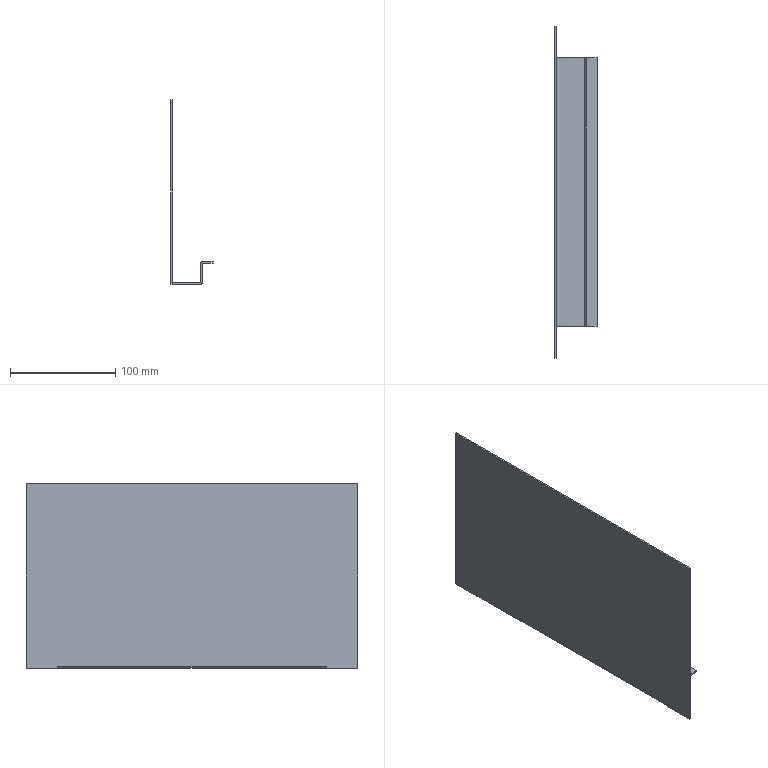Part | 1 solid | 38 faces | box 40 x 315 x 175 mm | volume 104644 mm3 | plane 32 | cylinder 6 | commonest cylinder face diameters 0.2 x3 3.2 x3
STEP:
#1=CARTESIAN_POINT('',(-217.5,127.5,-155.));
#2=VERTEX_POINT('',#1);
#3=CARTESIAN_POINT('',(-217.5,127.5,-153.5));
#4=VERTEX_POINT('',#3);
#5=CARTESIAN_POINT('',(-217.5,127.5,-663.884));
#6=DIRECTION('',(0.,0.,1.));
#7=VECTOR('',#6,1000.);
#8=LINE('',#5,#7);
#9=EDGE_CURVE('',#2,#4,#8,.T.);
#10=ORIENTED_EDGE('',*,*,#9,.T.);
#11=CARTESIAN_POINT('',(-217.5,-127.5,-153.5));
#12=VERTEX_POINT('',#11);
#13=CARTESIAN_POINT('',(-217.5,-127.5,-153.5));
#14=DIRECTION('',(0.,-1.,0.));
#15=VECTOR('',#14,1000.);
#16=LINE('',#13,#15);
#17=EDGE_CURVE('',#4,#12,#16,.T.);
#18=ORIENTED_EDGE('',*,*,#17,.T.);
#19=CARTESIAN_POINT('',(-217.5,-127.5,-155.));
#20=VERTEX_POINT('',#19);
#21=CARTESIAN_POINT('',(-217.5,-127.5,-663.884));
#22=DIRECTION('',(0.,0.,1.));
#23=VECTOR('',#22,1000.);
#24=LINE('',#21,#23);
#25=EDGE_CURVE('',#20,#12,#24,.T.);
#26=ORIENTED_EDGE('',*,*,#25,.F.);
#27=CARTESIAN_POINT('',(-217.5,-127.5,-155.));
#28=DIRECTION('',(0.,-1.,0.));
#29=VECTOR('',#28,1000.);
#30=LINE('',#27,#29);
#31=EDGE_CURVE('',#2,#20,#30,.T.);
#32=ORIENTED_EDGE('',*,*,#31,.F.);
#33=EDGE_LOOP('',(#10,#18,#26,#32));
#34=FACE_OUTER_BOUND('',#33,.T.);
#35=CARTESIAN_POINT('',(-217.5,-127.5,-663.884));
#36=DIRECTION('',(-1.,0.,0.));
#37=DIRECTION('',(0.,-1.,0.));
#38=AXIS2_PLACEMENT_3D('',#35,#36,#37);
#39=PLANE('',#38);
#40=ADVANCED_FACE('',(#34),#39,.F.);
#41=CARTESIAN_POINT('',(-227.4,127.5,-153.5));
#42=VERTEX_POINT('',#41);
#43=CARTESIAN_POINT('',(-2832.5,127.5,-153.5));
#44=DIRECTION('',(-1.,0.,0.));
#45=VECTOR('',#44,1000.);
#46=LINE('',#43,#45);
#47=EDGE_CURVE('',#4,#42,#46,.T.);
#48=ORIENTED_EDGE('',*,*,#47,.F.);
#49=ORIENTED_EDGE('',*,*,#9,.F.);
#50=CARTESIAN_POINT('',(-227.4,127.5,-155.));
#51=VERTEX_POINT('',#50);
#52=CARTESIAN_POINT('',(2832.5,127.5,-155.));
#53=DIRECTION('',(-1.,0.,0.));
#54=VECTOR('',#53,1000.);
#55=LINE('',#52,#54);
#56=EDGE_CURVE('',#2,#51,#55,.T.);
#57=ORIENTED_EDGE('',*,*,#56,.T.);
#58=CARTESIAN_POINT('',(-227.4,127.5,-663.884));
#59=DIRECTION('',(0.,0.,1.));
#60=VECTOR('',#59,1000.);
#61=LINE('',#58,#60);
#62=EDGE_CURVE('',#51,#42,#61,.T.);
#63=ORIENTED_EDGE('',*,*,#62,.T.);
#64=EDGE_LOOP('',(#48,#49,#57,#63));
#65=FACE_OUTER_BOUND('',#64,.T.);
#66=CARTESIAN_POINT('',(2832.5,127.5,-663.884));
#67=DIRECTION('',(0.,1.,0.));
#68=DIRECTION('',(-1.,0.,0.));
#69=AXIS2_PLACEMENT_3D('',#66,#67,#68);
#70=PLANE('',#69);
#71=ADVANCED_FACE('',(#65),#70,.T.);
#72=ORIENTED_EDGE('',*,*,#47,.T.);
#73=CARTESIAN_POINT('',(-227.4,-127.5,-153.5));
#74=VERTEX_POINT('',#73);
#75=CARTESIAN_POINT('',(-227.4,127.5,-153.5));
#76=DIRECTION('',(0.,-1.,0.));
#77=VECTOR('',#76,1000.);
#78=LINE('',#75,#77);
#79=EDGE_CURVE('',#42,#74,#78,.T.);
#80=ORIENTED_EDGE('',*,*,#79,.T.);
#81=CARTESIAN_POINT('',(-2832.5,-127.5,-153.5));
#82=DIRECTION('',(1.,0.,0.));
#83=VECTOR('',#82,1000.);
#84=LINE('',#81,#83);
#85=EDGE_CURVE('',#74,#12,#84,.T.);
#86=ORIENTED_EDGE('',*,*,#85,.T.);
#87=ORIENTED_EDGE('',*,*,#17,.F.);
#88=EDGE_LOOP('',(#72,#80,#86,#87));
#89=FACE_OUTER_BOUND('',#88,.T.);
#90=CARTESIAN_POINT('',(-2832.5,-127.5,-153.5));
#91=DIRECTION('',(0.,0.,-1.));
#92=DIRECTION('',(0.,-1.,0.));
#93=AXIS2_PLACEMENT_3D('',#90,#91,#92);
#94=PLANE('',#93);
#95=ADVANCED_FACE('',(#89),#94,.F.);
#96=ORIENTED_EDGE('',*,*,#85,.F.);
#97=CARTESIAN_POINT('',(-227.4,-127.5,-155.));
#98=VERTEX_POINT('',#97);
#99=CARTESIAN_POINT('',(-227.4,-127.5,-663.884));
#100=DIRECTION('',(0.,0.,1.));
#101=VECTOR('',#100,1000.);
#102=LINE('',#99,#101);
#103=EDGE_CURVE('',#98,#74,#102,.T.);
#104=ORIENTED_EDGE('',*,*,#103,.F.);
#105=CARTESIAN_POINT('',(-2832.5,-127.5,-155.));
#106=DIRECTION('',(1.,0.,0.));
#107=VECTOR('',#106,1000.);
#108=LINE('',#105,#107);
#109=EDGE_CURVE('',#98,#20,#108,.T.);
#110=ORIENTED_EDGE('',*,*,#109,.T.);
#111=ORIENTED_EDGE('',*,*,#25,.T.);
#112=EDGE_LOOP('',(#96,#104,#110,#111));
#113=FACE_OUTER_BOUND('',#112,.T.);
#114=CARTESIAN_POINT('',(-2832.5,-127.5,-663.884));
#115=DIRECTION('',(0.,-1.,0.));
#116=DIRECTION('',(1.,0.,0.));
#117=AXIS2_PLACEMENT_3D('',#114,#115,#116);
#118=PLANE('',#117);
#119=ADVANCED_FACE('',(#113),#118,.T.);
#120=CARTESIAN_POINT('',(-227.4,127.5,-155.));
#121=DIRECTION('',(0.,-1.,0.));
#122=VECTOR('',#121,1000.);
#123=LINE('',#120,#122);
#124=EDGE_CURVE('',#51,#98,#123,.T.);
#125=ORIENTED_EDGE('',*,*,#124,.F.);
#126=ORIENTED_EDGE('',*,*,#56,.F.);
#127=ORIENTED_EDGE('',*,*,#31,.T.);
#128=ORIENTED_EDGE('',*,*,#109,.F.);
#129=EDGE_LOOP('',(#125,#126,#127,#128));
#130=FACE_OUTER_BOUND('',#129,.T.);
#131=CARTESIAN_POINT('',(-2832.5,-127.5,-155.));
#132=DIRECTION('',(0.,0.,-1.));
#133=DIRECTION('',(0.,-1.,0.));
#134=AXIS2_PLACEMENT_3D('',#131,#132,#133);
#135=PLANE('',#134);
#136=ADVANCED_FACE('',(#130),#135,.T.);
#137=CARTESIAN_POINT('',(-227.5,127.5,-173.4));
#138=VERTEX_POINT('',#137);
#139=CARTESIAN_POINT('',(-227.5,127.5,-155.1));
#140=VERTEX_POINT('',#139);
#141=CARTESIAN_POINT('',(-227.5,127.5,-155.));
#142=DIRECTION('',(0.,0.,1.));
#143=VECTOR('',#142,1000.);
#144=LINE('',#141,#143);
#145=EDGE_CURVE('',#138,#140,#144,.T.);
#146=ORIENTED_EDGE('',*,*,#145,.F.);
#147=CARTESIAN_POINT('',(-229.,127.5,-173.4));
#148=VERTEX_POINT('',#147);
#149=CARTESIAN_POINT('',(-740.312,127.5,-173.4));
#150=DIRECTION('',(1.,0.,0.));
#151=VECTOR('',#150,1000.);
#152=LINE('',#149,#151);
#153=EDGE_CURVE('',#148,#138,#152,.T.);
#154=ORIENTED_EDGE('',*,*,#153,.F.);
#155=CARTESIAN_POINT('',(-229.,127.5,-155.1));
#156=VERTEX_POINT('',#155);
#157=CARTESIAN_POINT('',(-229.,127.5,-175.));
#158=DIRECTION('',(0.,0.,-1.));
#159=VECTOR('',#158,1000.);
#160=LINE('',#157,#159);
#161=EDGE_CURVE('',#156,#148,#160,.T.);
#162=ORIENTED_EDGE('',*,*,#161,.F.);
#163=CARTESIAN_POINT('',(-740.312,127.5,-155.1));
#164=DIRECTION('',(1.,0.,0.));
#165=VECTOR('',#164,1000.);
#166=LINE('',#163,#165);
#167=EDGE_CURVE('',#156,#140,#166,.T.);
#168=ORIENTED_EDGE('',*,*,#167,.T.);
#169=EDGE_LOOP('',(#146,#154,#162,#168));
#170=FACE_OUTER_BOUND('',#169,.T.);
#171=CARTESIAN_POINT('',(-740.312,127.5,-175.));
#172=DIRECTION('',(0.,-1.,0.));
#173=DIRECTION('',(0.,0.,1.));
#174=AXIS2_PLACEMENT_3D('',#171,#172,#173);
#175=PLANE('',#174);
#176=ADVANCED_FACE('',(#170),#175,.F.);
#177=CARTESIAN_POINT('',(-227.5,-127.5,-155.1));
#178=VERTEX_POINT('',#177);
#179=CARTESIAN_POINT('',(-227.5,-127.5,-173.4));
#180=VERTEX_POINT('',#179);
#181=CARTESIAN_POINT('',(-227.5,-127.5,-175.));
#182=DIRECTION('',(0.,0.,-1.));
#183=VECTOR('',#182,1000.);
#184=LINE('',#181,#183);
#185=EDGE_CURVE('',#178,#180,#184,.T.);
#186=ORIENTED_EDGE('',*,*,#185,.F.);
#187=CARTESIAN_POINT('',(-229.,-127.5,-155.1));
#188=VERTEX_POINT('',#187);
#189=CARTESIAN_POINT('',(-740.312,-127.5,-155.1));
#190=DIRECTION('',(1.,0.,0.));
#191=VECTOR('',#190,1000.);
#192=LINE('',#189,#191);
#193=EDGE_CURVE('',#188,#178,#192,.T.);
#194=ORIENTED_EDGE('',*,*,#193,.F.);
#195=CARTESIAN_POINT('',(-229.,-127.5,-173.4));
#196=VERTEX_POINT('',#195);
#197=CARTESIAN_POINT('',(-229.,-127.5,-175.));
#198=DIRECTION('',(0.,0.,-1.));
#199=VECTOR('',#198,1000.);
#200=LINE('',#197,#199);
#201=EDGE_CURVE('',#188,#196,#200,.T.);
#202=ORIENTED_EDGE('',*,*,#201,.T.);
#203=CARTESIAN_POINT('',(-740.312,-127.5,-173.4));
#204=DIRECTION('',(1.,0.,0.));
#205=VECTOR('',#204,1000.);
#206=LINE('',#203,#205);
#207=EDGE_CURVE('',#196,#180,#206,.T.);
#208=ORIENTED_EDGE('',*,*,#207,.T.);
#209=EDGE_LOOP('',(#186,#194,#202,#208));
#210=FACE_OUTER_BOUND('',#209,.T.);
#211=CARTESIAN_POINT('',(-740.312,-127.5,-175.));
#212=DIRECTION('',(0.,1.,0.));
#213=DIRECTION('',(0.,0.,-1.));
#214=AXIS2_PLACEMENT_3D('',#211,#212,#213);
#215=PLANE('',#214);
#216=ADVANCED_FACE('',(#210),#215,.F.);
#217=ORIENTED_EDGE('',*,*,#201,.F.);
#218=CARTESIAN_POINT('',(-229.,127.5,-155.1));
#219=DIRECTION('',(0.,1.,0.));
#220=VECTOR('',#219,1000.);
#221=LINE('',#218,#220);
#222=EDGE_CURVE('',#188,#156,#221,.T.);
#223=ORIENTED_EDGE('',*,*,#222,.T.);
#224=ORIENTED_EDGE('',*,*,#161,.T.);
#225=CARTESIAN_POINT('',(-229.,-127.5,-173.4));
#226=DIRECTION('',(0.,-1.,0.));
#227=VECTOR('',#226,1000.);
#228=LINE('',#225,#227);
#229=EDGE_CURVE('',#148,#196,#228,.T.);
#230=ORIENTED_EDGE('',*,*,#229,.T.);
#231=EDGE_LOOP('',(#217,#223,#224,#230));
#232=FACE_OUTER_BOUND('',#231,.T.);
#233=CARTESIAN_POINT('',(-229.,2732.5,-175.));
#234=DIRECTION('',(1.,0.,0.));
#235=DIRECTION('',(0.,0.,-1.));
#236=AXIS2_PLACEMENT_3D('',#233,#234,#235);
#237=PLANE('',#236);
#238=ADVANCED_FACE('',(#232),#237,.F.);
#239=CARTESIAN_POINT('',(-227.5,127.5,-155.1));
#240=DIRECTION('',(0.,1.,0.));
#241=VECTOR('',#240,1000.);
#242=LINE('',#239,#241);
#243=EDGE_CURVE('',#178,#140,#242,.T.);
#244=ORIENTED_EDGE('',*,*,#243,.F.);
#245=ORIENTED_EDGE('',*,*,#185,.T.);
#246=CARTESIAN_POINT('',(-227.5,-127.5,-173.4));
#247=DIRECTION('',(0.,-1.,0.));
#248=VECTOR('',#247,1000.);
#249=LINE('',#246,#248);
#250=EDGE_CURVE('',#138,#180,#249,.T.);
#251=ORIENTED_EDGE('',*,*,#250,.F.);
#252=ORIENTED_EDGE('',*,*,#145,.T.);
#253=EDGE_LOOP('',(#244,#245,#251,#252));
#254=FACE_OUTER_BOUND('',#253,.T.);
#255=CARTESIAN_POINT('',(-227.5,-127.5,-155.));
#256=DIRECTION('',(1.,0.,0.));
#257=DIRECTION('',(0.,0.,-1.));
#258=AXIS2_PLACEMENT_3D('',#255,#256,#257);
#259=PLANE('',#258);
#260=ADVANCED_FACE('',(#254),#259,.T.);
#261=CARTESIAN_POINT('',(-256.,-127.65,-173.25));
#262=VERTEX_POINT('',#261);
#263=CARTESIAN_POINT('',(-257.5,-127.65,-173.25));
#264=VERTEX_POINT('',#263);
#265=CARTESIAN_POINT('',(464.694,-127.65,-173.25));
#266=DIRECTION('',(-1.,0.,0.));
#267=VECTOR('',#266,1000.);
#268=LINE('',#265,#267);
#269=EDGE_CURVE('',#262,#264,#268,.T.);
#270=ORIENTED_EDGE('',*,*,#269,.T.);
#271=CARTESIAN_POINT('',(-257.5,-127.5,-173.25));
#272=VERTEX_POINT('',#271);
#273=CARTESIAN_POINT('',(-257.5,2732.5,-173.25));
#274=DIRECTION('',(0.,1.,0.));
#275=VECTOR('',#274,1000.);
#276=LINE('',#273,#275);
#277=EDGE_CURVE('',#264,#272,#276,.T.);
#278=ORIENTED_EDGE('',*,*,#277,.T.);
#279=CARTESIAN_POINT('',(-256.,-127.5,-173.25));
#280=VERTEX_POINT('',#279);
#281=CARTESIAN_POINT('',(464.694,-127.5,-173.25));
#282=DIRECTION('',(-1.,0.,0.));
#283=VECTOR('',#282,1000.);
#284=LINE('',#281,#283);
#285=EDGE_CURVE('',#280,#272,#284,.T.);
#286=ORIENTED_EDGE('',*,*,#285,.F.);
#287=CARTESIAN_POINT('',(-256.,2732.5,-173.25));
#288=DIRECTION('',(0.,1.,0.));
#289=VECTOR('',#288,1000.);
#290=LINE('',#287,#289);
#291=EDGE_CURVE('',#262,#280,#290,.T.);
#292=ORIENTED_EDGE('',*,*,#291,.F.);
#293=EDGE_LOOP('',(#270,#278,#286,#292));
#294=FACE_OUTER_BOUND('',#293,.T.);
#295=CARTESIAN_POINT('',(464.694,2732.5,-173.25));
#296=DIRECTION('',(0.,0.,1.));
#297=DIRECTION('',(0.,-1.,0.));
#298=AXIS2_PLACEMENT_3D('',#295,#296,#297);
#299=PLANE('',#298);
#300=ADVANCED_FACE('',(#294),#299,.F.);
#301=CARTESIAN_POINT('',(-256.,-127.65,-175.));
#302=VERTEX_POINT('',#301);
#303=CARTESIAN_POINT('',(-257.5,-127.65,-175.));
#304=VERTEX_POINT('',#303);
#305=CARTESIAN_POINT('',(464.694,-127.65,-175.));
#306=DIRECTION('',(-1.,0.,0.));
#307=VECTOR('',#306,1000.);
#308=LINE('',#305,#307);
#309=EDGE_CURVE('',#302,#304,#308,.T.);
#310=ORIENTED_EDGE('',*,*,#309,.T.);
#311=CARTESIAN_POINT('',(-257.5,-127.65,-173.063));
#312=DIRECTION('',(0.,0.,1.));
#313=VECTOR('',#312,1000.);
#314=LINE('',#311,#313);
#315=EDGE_CURVE('',#304,#264,#314,.T.);
#316=ORIENTED_EDGE('',*,*,#315,.T.);
#317=ORIENTED_EDGE('',*,*,#269,.F.);
#318=CARTESIAN_POINT('',(-256.,-127.65,-173.063));
#319=DIRECTION('',(0.,0.,1.));
#320=VECTOR('',#319,1000.);
#321=LINE('',#318,#320);
#322=EDGE_CURVE('',#302,#262,#321,.T.);
#323=ORIENTED_EDGE('',*,*,#322,.F.);
#324=EDGE_LOOP('',(#310,#316,#317,#323));
#325=FACE_OUTER_BOUND('',#324,.T.);
#326=CARTESIAN_POINT('',(464.694,-127.65,-173.063));
#327=DIRECTION('',(0.,-1.,0.));
#328=DIRECTION('',(0.,0.,-1.));
#329=AXIS2_PLACEMENT_3D('',#326,#327,#328);
#330=PLANE('',#329);
#331=ADVANCED_FACE('',(#325),#330,.F.);
#332=CARTESIAN_POINT('',(-257.5,-157.5,-175.));
#333=VERTEX_POINT('',#332);
#334=CARTESIAN_POINT('',(-257.5,2732.5,-175.));
#335=DIRECTION('',(0.,-1.,0.));
#336=VECTOR('',#335,1000.);
#337=LINE('',#334,#336);
#338=EDGE_CURVE('',#304,#333,#337,.T.);
#339=ORIENTED_EDGE('',*,*,#338,.F.);
#340=ORIENTED_EDGE('',*,*,#309,.F.);
#341=CARTESIAN_POINT('',(-256.,-157.5,-175.));
#342=VERTEX_POINT('',#341);
#343=CARTESIAN_POINT('',(-256.,2732.5,-175.));
#344=DIRECTION('',(0.,-1.,0.));
#345=VECTOR('',#344,1000.);
#346=LINE('',#343,#345);
#347=EDGE_CURVE('',#302,#342,#346,.T.);
#348=ORIENTED_EDGE('',*,*,#347,.T.);
#349=CARTESIAN_POINT('',(464.694,-157.5,-175.));
#350=DIRECTION('',(-1.,0.,0.));
#351=VECTOR('',#350,1000.);
#352=LINE('',#349,#351);
#353=EDGE_CURVE('',#342,#333,#352,.T.);
#354=ORIENTED_EDGE('',*,*,#353,.T.);
#355=EDGE_LOOP('',(#339,#340,#348,#354));
#356=FACE_OUTER_BOUND('',#355,.T.);
#357=CARTESIAN_POINT('',(464.694,2732.5,-175.));
#358=DIRECTION('',(0.,0.,-1.));
#359=DIRECTION('',(-1.,0.,0.));
#360=AXIS2_PLACEMENT_3D('',#357,#358,#359);
#361=PLANE('',#360);
#362=ADVANCED_FACE('',(#356),#361,.T.);
#363=CARTESIAN_POINT('',(-256.,-157.5,0.));
#364=VERTEX_POINT('',#363);
#365=CARTESIAN_POINT('',(-257.5,-157.5,0.));
#366=VERTEX_POINT('',#365);
#367=CARTESIAN_POINT('',(464.694,-157.5,0.));
#368=DIRECTION('',(-1.,0.,0.));
#369=VECTOR('',#368,1000.);
#370=LINE('',#367,#369);
#371=EDGE_CURVE('',#364,#366,#370,.T.);
#372=ORIENTED_EDGE('',*,*,#371,.T.);
#373=CARTESIAN_POINT('',(-257.5,-157.5,-173.063));
#374=DIRECTION('',(0.,0.,-1.));
#375=VECTOR('',#374,1000.);
#376=LINE('',#373,#375);
#377=EDGE_CURVE('',#366,#333,#376,.T.);
#378=ORIENTED_EDGE('',*,*,#377,.T.);
#379=ORIENTED_EDGE('',*,*,#353,.F.);
#380=CARTESIAN_POINT('',(-256.,-157.5,-173.063));
#381=DIRECTION('',(0.,0.,-1.));
#382=VECTOR('',#381,1000.);
#383=LINE('',#380,#382);
#384=EDGE_CURVE('',#364,#342,#383,.T.);
#385=ORIENTED_EDGE('',*,*,#384,.F.);
#386=EDGE_LOOP('',(#372,#378,#379,#385));
#387=FACE_OUTER_BOUND('',#386,.T.);
#388=CARTESIAN_POINT('',(464.694,-157.5,-173.063));
#389=DIRECTION('',(0.,1.,0.));
#390=DIRECTION('',(-1.,0.,0.));
#391=AXIS2_PLACEMENT_3D('',#388,#389,#390);
#392=PLANE('',#391);
#393=ADVANCED_FACE('',(#387),#392,.F.);
#394=CARTESIAN_POINT('',(-257.5,157.5,0.));
#395=VERTEX_POINT('',#394);
#396=CARTESIAN_POINT('',(-257.5,2732.5,0.));
#397=DIRECTION('',(0.,-1.,0.));
#398=VECTOR('',#397,1000.);
#399=LINE('',#396,#398);
#400=EDGE_CURVE('',#395,#366,#399,.T.);
#401=ORIENTED_EDGE('',*,*,#400,.T.);
#402=ORIENTED_EDGE('',*,*,#371,.F.);
#403=CARTESIAN_POINT('',(-256.,157.5,0.));
#404=VERTEX_POINT('',#403);
#405=CARTESIAN_POINT('',(-256.,0.,0.));
#406=DIRECTION('',(0.,1.,0.));
#407=VECTOR('',#406,1000.);
#408=LINE('',#405,#407);
#409=EDGE_CURVE('',#364,#404,#408,.T.);
#410=ORIENTED_EDGE('',*,*,#409,.T.);
#411=CARTESIAN_POINT('',(464.694,157.5,0.));
#412=DIRECTION('',(-1.,0.,0.));
#413=VECTOR('',#412,1000.);
#414=LINE('',#411,#413);
#415=EDGE_CURVE('',#404,#395,#414,.T.);
#416=ORIENTED_EDGE('',*,*,#415,.T.);
#417=EDGE_LOOP('',(#401,#402,#410,#416));
#418=FACE_OUTER_BOUND('',#417,.T.);
#419=CARTESIAN_POINT('',(464.694,0.,0.));
#420=DIRECTION('',(0.,0.,1.));
#421=DIRECTION('',(1.,0.,0.));
#422=AXIS2_PLACEMENT_3D('',#419,#420,#421);
#423=PLANE('',#422);
#424=ADVANCED_FACE('',(#418),#423,.T.);
#425=CARTESIAN_POINT('',(-256.,157.5,-175.));
#426=VERTEX_POINT('',#425);
#427=CARTESIAN_POINT('',(-257.5,157.5,-175.));
#428=VERTEX_POINT('',#427);
#429=CARTESIAN_POINT('',(464.694,157.5,-175.));
#430=DIRECTION('',(-1.,0.,0.));
#431=VECTOR('',#430,1000.);
#432=LINE('',#429,#431);
#433=EDGE_CURVE('',#426,#428,#432,.T.);
#434=ORIENTED_EDGE('',*,*,#433,.T.);
#435=CARTESIAN_POINT('',(-257.5,157.5,-173.063));
#436=DIRECTION('',(0.,0.,-1.));
#437=VECTOR('',#436,1000.);
#438=LINE('',#435,#437);
#439=EDGE_CURVE('',#395,#428,#438,.T.);
#440=ORIENTED_EDGE('',*,*,#439,.F.);
#441=ORIENTED_EDGE('',*,*,#415,.F.);
#442=CARTESIAN_POINT('',(-256.,157.5,-173.063));
#443=DIRECTION('',(0.,0.,1.));
#444=VECTOR('',#443,1000.);
#445=LINE('',#442,#444);
#446=EDGE_CURVE('',#426,#404,#445,.T.);
#447=ORIENTED_EDGE('',*,*,#446,.F.);
#448=EDGE_LOOP('',(#434,#440,#441,#447));
#449=FACE_OUTER_BOUND('',#448,.T.);
#450=CARTESIAN_POINT('',(464.694,157.5,-173.063));
#451=DIRECTION('',(0.,-1.,0.));
#452=DIRECTION('',(1.,0.,0.));
#453=AXIS2_PLACEMENT_3D('',#450,#451,#452);
#454=PLANE('',#453);
#455=ADVANCED_FACE('',(#449),#454,.F.);
#456=CARTESIAN_POINT('',(-257.5,127.65,-175.));
#457=VERTEX_POINT('',#456);
#458=CARTESIAN_POINT('',(-257.5,2732.5,-175.));
#459=DIRECTION('',(0.,-1.,0.));
#460=VECTOR('',#459,1000.);
#461=LINE('',#458,#460);
#462=EDGE_CURVE('',#428,#457,#461,.T.);
#463=ORIENTED_EDGE('',*,*,#462,.F.);
#464=ORIENTED_EDGE('',*,*,#433,.F.);
#465=CARTESIAN_POINT('',(-256.,127.65,-175.));
#466=VERTEX_POINT('',#465);
#467=CARTESIAN_POINT('',(-256.,2732.5,-175.));
#468=DIRECTION('',(0.,-1.,0.));
#469=VECTOR('',#468,1000.);
#470=LINE('',#467,#469);
#471=EDGE_CURVE('',#426,#466,#470,.T.);
#472=ORIENTED_EDGE('',*,*,#471,.T.);
#473=CARTESIAN_POINT('',(464.694,127.65,-175.));
#474=DIRECTION('',(-1.,0.,0.));
#475=VECTOR('',#474,1000.);
#476=LINE('',#473,#475);
#477=EDGE_CURVE('',#466,#457,#476,.T.);
#478=ORIENTED_EDGE('',*,*,#477,.T.);
#479=EDGE_LOOP('',(#463,#464,#472,#478));
#480=FACE_OUTER_BOUND('',#479,.T.);
#481=CARTESIAN_POINT('',(464.694,2732.5,-175.));
#482=DIRECTION('',(0.,0.,-1.));
#483=DIRECTION('',(-1.,0.,0.));
#484=AXIS2_PLACEMENT_3D('',#481,#482,#483);
#485=PLANE('',#484);
#486=ADVANCED_FACE('',(#480),#485,.T.);
#487=CARTESIAN_POINT('',(-256.,127.65,-173.25));
#488=VERTEX_POINT('',#487);
#489=CARTESIAN_POINT('',(-257.5,127.65,-173.25));
#490=VERTEX_POINT('',#489);
#491=CARTESIAN_POINT('',(464.694,127.65,-173.25));
#492=DIRECTION('',(-1.,0.,0.));
#493=VECTOR('',#492,1000.);
#494=LINE('',#491,#493);
#495=EDGE_CURVE('',#488,#490,#494,.T.);
#496=ORIENTED_EDGE('',*,*,#495,.T.);
#497=CARTESIAN_POINT('',(-257.5,127.65,-173.063));
#498=DIRECTION('',(0.,0.,-1.));
#499=VECTOR('',#498,1000.);
#500=LINE('',#497,#499);
#501=EDGE_CURVE('',#490,#457,#500,.T.);
#502=ORIENTED_EDGE('',*,*,#501,.T.);
#503=ORIENTED_EDGE('',*,*,#477,.F.);
#504=CARTESIAN_POINT('',(-256.,127.65,-173.063));
#505=DIRECTION('',(0.,0.,-1.));
#506=VECTOR('',#505,1000.);
#507=LINE('',#504,#506);
#508=EDGE_CURVE('',#488,#466,#507,.T.);
#509=ORIENTED_EDGE('',*,*,#508,.F.);
#510=EDGE_LOOP('',(#496,#502,#503,#509));
#511=FACE_OUTER_BOUND('',#510,.T.);
#512=CARTESIAN_POINT('',(464.694,127.65,-173.063));
#513=DIRECTION('',(0.,1.,0.));
#514=DIRECTION('',(0.,0.,1.));
#515=AXIS2_PLACEMENT_3D('',#512,#513,#514);
#516=PLANE('',#515);
#517=ADVANCED_FACE('',(#511),#516,.F.);
#518=CARTESIAN_POINT('',(-256.,127.5,-173.25));
#519=VERTEX_POINT('',#518);
#520=CARTESIAN_POINT('',(-257.5,127.5,-173.25));
#521=VERTEX_POINT('',#520);
#522=CARTESIAN_POINT('',(464.694,127.5,-173.25));
#523=DIRECTION('',(-1.,0.,0.));
#524=VECTOR('',#523,1000.);
#525=LINE('',#522,#524);
#526=EDGE_CURVE('',#519,#521,#525,.T.);
#527=ORIENTED_EDGE('',*,*,#526,.T.);
#528=CARTESIAN_POINT('',(-257.5,2732.5,-173.25));
#529=DIRECTION('',(0.,1.,0.));
#530=VECTOR('',#529,1000.);
#531=LINE('',#528,#530);
#532=EDGE_CURVE('',#521,#490,#531,.T.);
#533=ORIENTED_EDGE('',*,*,#532,.T.);
#534=ORIENTED_EDGE('',*,*,#495,.F.);
#535=CARTESIAN_POINT('',(-256.,2732.5,-173.25));
#536=DIRECTION('',(0.,1.,0.));
#537=VECTOR('',#536,1000.);
#538=LINE('',#535,#537);
#539=EDGE_CURVE('',#519,#488,#538,.T.);
#540=ORIENTED_EDGE('',*,*,#539,.F.);
#541=EDGE_LOOP('',(#527,#533,#534,#540));
#542=FACE_OUTER_BOUND('',#541,.T.);
#543=CARTESIAN_POINT('',(464.694,2732.5,-173.25));
#544=DIRECTION('',(0.,0.,1.));
#545=DIRECTION('',(0.,-1.,0.));
#546=AXIS2_PLACEMENT_3D('',#543,#544,#545);
#547=PLANE('',#546);
#548=ADVANCED_FACE('',(#542),#547,.F.);
#549=ORIENTED_EDGE('',*,*,#285,.T.);
#550=CARTESIAN_POINT('',(-257.5,-127.5,-173.4));
#551=VERTEX_POINT('',#550);
#552=CARTESIAN_POINT('',(-257.5,-127.5,-173.063));
#553=DIRECTION('',(0.,0.,-1.));
#554=VECTOR('',#553,1000.);
#555=LINE('',#552,#554);
#556=EDGE_CURVE('',#272,#551,#555,.T.);
#557=ORIENTED_EDGE('',*,*,#556,.T.);
#558=CARTESIAN_POINT('',(-256.,-127.5,-173.4));
#559=VERTEX_POINT('',#558);
#560=CARTESIAN_POINT('',(464.694,-127.5,-173.4));
#561=DIRECTION('',(-1.,0.,0.));
#562=VECTOR('',#561,1000.);
#563=LINE('',#560,#562);
#564=EDGE_CURVE('',#559,#551,#563,.T.);
#565=ORIENTED_EDGE('',*,*,#564,.F.);
#566=CARTESIAN_POINT('',(-256.,-127.5,-173.063));
#567=DIRECTION('',(0.,0.,-1.));
#568=VECTOR('',#567,1000.);
#569=LINE('',#566,#568);
#570=EDGE_CURVE('',#280,#559,#569,.T.);
#571=ORIENTED_EDGE('',*,*,#570,.F.);
#572=EDGE_LOOP('',(#549,#557,#565,#571));
#573=FACE_OUTER_BOUND('',#572,.T.);
#574=CARTESIAN_POINT('',(464.694,-127.5,-173.063));
#575=DIRECTION('',(0.,1.,0.));
#576=DIRECTION('',(0.,0.,1.));
#577=AXIS2_PLACEMENT_3D('',#574,#575,#576);
#578=PLANE('',#577);
#579=ADVANCED_FACE('',(#573),#578,.F.);
#580=CARTESIAN_POINT('',(-257.5,127.5,-173.4));
#581=VERTEX_POINT('',#580);
#582=CARTESIAN_POINT('',(-257.5,-127.5,-173.4));
#583=DIRECTION('',(0.,1.,0.));
#584=VECTOR('',#583,1000.);
#585=LINE('',#582,#584);
#586=EDGE_CURVE('',#551,#581,#585,.T.);
#587=ORIENTED_EDGE('',*,*,#586,.F.);
#588=ORIENTED_EDGE('',*,*,#556,.F.);
#589=ORIENTED_EDGE('',*,*,#277,.F.);
#590=ORIENTED_EDGE('',*,*,#315,.F.);
#591=ORIENTED_EDGE('',*,*,#338,.T.);
#592=ORIENTED_EDGE('',*,*,#377,.F.);
#593=ORIENTED_EDGE('',*,*,#400,.F.);
#594=ORIENTED_EDGE('',*,*,#439,.T.);
#595=ORIENTED_EDGE('',*,*,#462,.T.);
#596=ORIENTED_EDGE('',*,*,#501,.F.);
#597=ORIENTED_EDGE('',*,*,#532,.F.);
#598=CARTESIAN_POINT('',(-257.5,127.5,-173.063));
#599=DIRECTION('',(0.,0.,1.));
#600=VECTOR('',#599,1000.);
#601=LINE('',#598,#600);
#602=EDGE_CURVE('',#581,#521,#601,.T.);
#603=ORIENTED_EDGE('',*,*,#602,.F.);
#604=EDGE_LOOP('',(#587,#588,#589,#590,#591,#592,#593,#594,#595,#596,#597,#603));
#605=FACE_OUTER_BOUND('',#604,.T.);
#606=CARTESIAN_POINT('',(-257.5,2732.5,-173.063));
#607=DIRECTION('',(1.,0.,0.));
#608=DIRECTION('',(0.,1.,0.));
#609=AXIS2_PLACEMENT_3D('',#606,#607,#608);
#610=PLANE('',#609);
#611=ADVANCED_FACE('',(#605),#610,.F.);
#612=CARTESIAN_POINT('',(-256.,127.5,-173.4));
#613=VERTEX_POINT('',#612);
#614=CARTESIAN_POINT('',(464.694,127.5,-173.4));
#615=DIRECTION('',(-1.,0.,0.));
#616=VECTOR('',#615,1000.);
#617=LINE('',#614,#616);
#618=EDGE_CURVE('',#613,#581,#617,.T.);
#619=ORIENTED_EDGE('',*,*,#618,.T.);
#620=ORIENTED_EDGE('',*,*,#602,.T.);
#621=ORIENTED_EDGE('',*,*,#526,.F.);
#622=CARTESIAN_POINT('',(-256.,127.5,-173.063));
#623=DIRECTION('',(0.,0.,1.));
#624=VECTOR('',#623,1000.);
#625=LINE('',#622,#624);
#626=EDGE_CURVE('',#613,#519,#625,.T.);
#627=ORIENTED_EDGE('',*,*,#626,.F.);
#628=EDGE_LOOP('',(#619,#620,#621,#627));
#629=FACE_OUTER_BOUND('',#628,.T.);
#630=CARTESIAN_POINT('',(464.694,127.5,-173.063));
#631=DIRECTION('',(0.,-1.,0.));
#632=DIRECTION('',(0.,0.,-1.));
#633=AXIS2_PLACEMENT_3D('',#630,#631,#632);
#634=PLANE('',#633);
#635=ADVANCED_FACE('',(#629),#634,.F.);
#636=ORIENTED_EDGE('',*,*,#570,.T.);
#637=CARTESIAN_POINT('',(-256.,-127.5,-173.4));
#638=DIRECTION('',(0.,1.,0.));
#639=VECTOR('',#638,1000.);
#640=LINE('',#637,#639);
#641=EDGE_CURVE('',#559,#613,#640,.T.);
#642=ORIENTED_EDGE('',*,*,#641,.T.);
#643=ORIENTED_EDGE('',*,*,#626,.T.);
#644=ORIENTED_EDGE('',*,*,#539,.T.);
#645=ORIENTED_EDGE('',*,*,#508,.T.);
#646=ORIENTED_EDGE('',*,*,#471,.F.);
#647=ORIENTED_EDGE('',*,*,#446,.T.);
#648=ORIENTED_EDGE('',*,*,#409,.F.);
#649=ORIENTED_EDGE('',*,*,#384,.T.);
#650=ORIENTED_EDGE('',*,*,#347,.F.);
#651=ORIENTED_EDGE('',*,*,#322,.T.);
#652=ORIENTED_EDGE('',*,*,#291,.T.);
#653=EDGE_LOOP('',(#636,#642,#643,#644,#645,#646,#647,#648,#649,#650,#651,#652));
#654=FACE_OUTER_BOUND('',#653,.T.);
#655=CARTESIAN_POINT('',(-256.,2732.5,-173.063));
#656=DIRECTION('',(1.,0.,0.));
#657=DIRECTION('',(0.,1.,0.));
#658=AXIS2_PLACEMENT_3D('',#655,#656,#657);
#659=PLANE('',#658);
#660=ADVANCED_FACE('',(#654),#659,.T.);
#661=CARTESIAN_POINT('',(-255.9,-127.5,-173.5));
#662=VERTEX_POINT('',#661);
#663=CARTESIAN_POINT('',(-255.9,-127.5,-175.));
#664=VERTEX_POINT('',#663);
#665=CARTESIAN_POINT('',(-255.9,-127.5,339.309));
#666=DIRECTION('',(0.,0.,-1.));
#667=VECTOR('',#666,1000.);
#668=LINE('',#665,#667);
#669=EDGE_CURVE('',#662,#664,#668,.T.);
#670=ORIENTED_EDGE('',*,*,#669,.F.);
#671=CARTESIAN_POINT('',(-255.9,-127.5,-173.4));
#672=DIRECTION('',(0.,1.,0.));
#673=DIRECTION('',(0.,0.,1.));
#674=AXIS2_PLACEMENT_3D('',#671,#672,#673);
#675=CIRCLE('',#674,0.1);
#676=EDGE_CURVE('',#662,#559,#675,.T.);
#677=ORIENTED_EDGE('',*,*,#676,.T.);
#678=ORIENTED_EDGE('',*,*,#564,.T.);
#679=CARTESIAN_POINT('',(-255.9,-127.5,-173.4));
#680=DIRECTION('',(0.,1.,0.));
#681=DIRECTION('',(0.,0.,1.));
#682=AXIS2_PLACEMENT_3D('',#679,#680,#681);
#683=CIRCLE('',#682,1.6);
#684=EDGE_CURVE('',#664,#551,#683,.T.);
#685=ORIENTED_EDGE('',*,*,#684,.F.);
#686=EDGE_LOOP('',(#670,#677,#678,#685));
#687=FACE_OUTER_BOUND('',#686,.T.);
#688=CARTESIAN_POINT('',(-255.9,-127.5,-173.4));
#689=DIRECTION('',(0.,-1.,0.));
#690=DIRECTION('',(0.,0.,-1.));
#691=AXIS2_PLACEMENT_3D('',#688,#689,#690);
#692=PLANE('',#691);
#693=ADVANCED_FACE('',(#687),#692,.T.);
#694=ORIENTED_EDGE('',*,*,#684,.T.);
#695=ORIENTED_EDGE('',*,*,#586,.T.);
#696=CARTESIAN_POINT('',(-255.9,127.5,-175.));
#697=VERTEX_POINT('',#696);
#698=CARTESIAN_POINT('',(-255.9,127.5,-173.4));
#699=DIRECTION('',(0.,-1.,0.));
#700=DIRECTION('',(0.,0.,1.));
#701=AXIS2_PLACEMENT_3D('',#698,#699,#700);
#702=CIRCLE('',#701,1.6);
#703=EDGE_CURVE('',#581,#697,#702,.T.);
#704=ORIENTED_EDGE('',*,*,#703,.T.);
#705=CARTESIAN_POINT('',(-255.9,-127.5,-175.));
#706=DIRECTION('',(0.,-1.,0.));
#707=VECTOR('',#706,1000.);
#708=LINE('',#705,#707);
#709=EDGE_CURVE('',#697,#664,#708,.T.);
#710=ORIENTED_EDGE('',*,*,#709,.T.);
#711=EDGE_LOOP('',(#694,#695,#704,#710));
#712=FACE_OUTER_BOUND('',#711,.T.);
#713=CARTESIAN_POINT('',(-255.9,-518.007,-173.4));
#714=DIRECTION('',(0.,1.,0.));
#715=DIRECTION('',(0.,0.,1.));
#716=AXIS2_PLACEMENT_3D('',#713,#714,#715);
#717=CYLINDRICAL_SURFACE('',#716,1.6);
#718=ADVANCED_FACE('',(#712),#717,.T.);
#719=ORIENTED_EDGE('',*,*,#618,.F.);
#720=CARTESIAN_POINT('',(-255.9,127.5,-173.5));
#721=VERTEX_POINT('',#720);
#722=CARTESIAN_POINT('',(-255.9,127.5,-173.4));
#723=DIRECTION('',(0.,-1.,0.));
#724=DIRECTION('',(0.,0.,1.));
#725=AXIS2_PLACEMENT_3D('',#722,#723,#724);
#726=CIRCLE('',#725,0.1);
#727=EDGE_CURVE('',#613,#721,#726,.T.);
#728=ORIENTED_EDGE('',*,*,#727,.T.);
#729=CARTESIAN_POINT('',(-255.9,127.5,339.309));
#730=DIRECTION('',(0.,0.,-1.));
#731=VECTOR('',#730,1000.);
#732=LINE('',#729,#731);
#733=EDGE_CURVE('',#721,#697,#732,.T.);
#734=ORIENTED_EDGE('',*,*,#733,.T.);
#735=ORIENTED_EDGE('',*,*,#703,.F.);
#736=EDGE_LOOP('',(#719,#728,#734,#735));
#737=FACE_OUTER_BOUND('',#736,.T.);
#738=CARTESIAN_POINT('',(-255.9,127.5,-173.4));
#739=DIRECTION('',(0.,1.,0.));
#740=DIRECTION('',(0.,0.,1.));
#741=AXIS2_PLACEMENT_3D('',#738,#739,#740);
#742=PLANE('',#741);
#743=ADVANCED_FACE('',(#737),#742,.T.);
#744=ORIENTED_EDGE('',*,*,#676,.F.);
#745=CARTESIAN_POINT('',(-255.9,-127.5,-173.5));
#746=DIRECTION('',(0.,-1.,0.));
#747=VECTOR('',#746,1000.);
#748=LINE('',#745,#747);
#749=EDGE_CURVE('',#721,#662,#748,.T.);
#750=ORIENTED_EDGE('',*,*,#749,.F.);
#751=ORIENTED_EDGE('',*,*,#727,.F.);
#752=ORIENTED_EDGE('',*,*,#641,.F.);
#753=EDGE_LOOP('',(#744,#750,#751,#752));
#754=FACE_OUTER_BOUND('',#753,.T.);
#755=CARTESIAN_POINT('',(-255.9,-518.007,-173.4));
#756=DIRECTION('',(0.,1.,0.));
#757=DIRECTION('',(0.,0.,1.));
#758=AXIS2_PLACEMENT_3D('',#755,#756,#757);
#759=CYLINDRICAL_SURFACE('',#758,0.1);
#760=ADVANCED_FACE('',(#754),#759,.F.);
#761=CARTESIAN_POINT('',(-229.1,127.5,-173.5));
#762=VERTEX_POINT('',#761);
#763=CARTESIAN_POINT('',(-229.1,-127.5,-173.5));
#764=VERTEX_POINT('',#763);
#765=CARTESIAN_POINT('',(-229.1,-127.5,-173.5));
#766=DIRECTION('',(0.,-1.,0.));
#767=VECTOR('',#766,1000.);
#768=LINE('',#765,#767);
#769=EDGE_CURVE('',#762,#764,#768,.T.);
#770=ORIENTED_EDGE('',*,*,#769,.F.);
#771=CARTESIAN_POINT('',(-2832.5,127.5,-173.5));
#772=DIRECTION('',(-1.,0.,0.));
#773=VECTOR('',#772,1000.);
#774=LINE('',#771,#773);
#775=EDGE_CURVE('',#762,#721,#774,.T.);
#776=ORIENTED_EDGE('',*,*,#775,.T.);
#777=ORIENTED_EDGE('',*,*,#749,.T.);
#778=CARTESIAN_POINT('',(-2832.5,-127.5,-173.5));
#779=DIRECTION('',(1.,0.,0.));
#780=VECTOR('',#779,1000.);
#781=LINE('',#778,#780);
#782=EDGE_CURVE('',#662,#764,#781,.T.);
#783=ORIENTED_EDGE('',*,*,#782,.T.);
#784=EDGE_LOOP('',(#770,#776,#777,#783));
#785=FACE_OUTER_BOUND('',#784,.T.);
#786=CARTESIAN_POINT('',(-2832.5,-157.5,-173.5));
#787=DIRECTION('',(0.,0.,-1.));
#788=DIRECTION('',(0.,-1.,0.));
#789=AXIS2_PLACEMENT_3D('',#786,#787,#788);
#790=PLANE('',#789);
#791=ADVANCED_FACE('',(#785),#790,.F.);
#792=CARTESIAN_POINT('',(-229.1,127.5,-175.));
#793=VERTEX_POINT('',#792);
#794=CARTESIAN_POINT('',(-257.5,127.5,-175.));
#795=DIRECTION('',(-1.,0.,0.));
#796=VECTOR('',#795,1000.);
#797=LINE('',#794,#796);
#798=EDGE_CURVE('',#793,#697,#797,.T.);
#799=ORIENTED_EDGE('',*,*,#798,.T.);
#800=ORIENTED_EDGE('',*,*,#733,.F.);
#801=ORIENTED_EDGE('',*,*,#775,.F.);
#802=CARTESIAN_POINT('',(-229.1,127.5,339.309));
#803=DIRECTION('',(0.,0.,-1.));
#804=VECTOR('',#803,1000.);
#805=LINE('',#802,#804);
#806=EDGE_CURVE('',#762,#793,#805,.T.);
#807=ORIENTED_EDGE('',*,*,#806,.T.);
#808=EDGE_LOOP('',(#799,#800,#801,#807));
#809=FACE_OUTER_BOUND('',#808,.T.);
#810=CARTESIAN_POINT('',(-2832.5,127.5,339.309));
#811=DIRECTION('',(0.,-1.,0.));
#812=DIRECTION('',(1.,0.,0.));
#813=AXIS2_PLACEMENT_3D('',#810,#811,#812);
#814=PLANE('',#813);
#815=ADVANCED_FACE('',(#809),#814,.F.);
#816=ORIENTED_EDGE('',*,*,#798,.F.);
#817=CARTESIAN_POINT('',(-229.1,-127.5,-175.));
#818=VERTEX_POINT('',#817);
#819=CARTESIAN_POINT('',(-229.1,-127.5,-175.));
#820=DIRECTION('',(0.,-1.,0.));
#821=VECTOR('',#820,1000.);
#822=LINE('',#819,#821);
#823=EDGE_CURVE('',#793,#818,#822,.T.);
#824=ORIENTED_EDGE('',*,*,#823,.T.);
#825=CARTESIAN_POINT('',(-257.5,-127.5,-175.));
#826=DIRECTION('',(1.,0.,0.));
#827=VECTOR('',#826,1000.);
#828=LINE('',#825,#827);
#829=EDGE_CURVE('',#664,#818,#828,.T.);
#830=ORIENTED_EDGE('',*,*,#829,.F.);
#831=ORIENTED_EDGE('',*,*,#709,.F.);
#832=EDGE_LOOP('',(#816,#824,#830,#831));
#833=FACE_OUTER_BOUND('',#832,.T.);
#834=CARTESIAN_POINT('',(-257.5,2732.5,-175.));
#835=DIRECTION('',(0.,0.,-1.));
#836=DIRECTION('',(-1.,0.,0.));
#837=AXIS2_PLACEMENT_3D('',#834,#835,#836);
#838=PLANE('',#837);
#839=ADVANCED_FACE('',(#833),#838,.T.);
#840=ORIENTED_EDGE('',*,*,#829,.T.);
#841=CARTESIAN_POINT('',(-229.1,-127.5,339.309));
#842=DIRECTION('',(0.,0.,-1.));
#843=VECTOR('',#842,1000.);
#844=LINE('',#841,#843);
#845=EDGE_CURVE('',#764,#818,#844,.T.);
#846=ORIENTED_EDGE('',*,*,#845,.F.);
#847=ORIENTED_EDGE('',*,*,#782,.F.);
#848=ORIENTED_EDGE('',*,*,#669,.T.);
#849=EDGE_LOOP('',(#840,#846,#847,#848));
#850=FACE_OUTER_BOUND('',#849,.T.);
#851=CARTESIAN_POINT('',(-2832.5,-127.5,339.309));
#852=DIRECTION('',(0.,1.,0.));
#853=DIRECTION('',(-1.,0.,0.));
#854=AXIS2_PLACEMENT_3D('',#851,#852,#853);
#855=PLANE('',#854);
#856=ADVANCED_FACE('',(#850),#855,.F.);
#857=ORIENTED_EDGE('',*,*,#207,.F.);
#858=CARTESIAN_POINT('',(-229.1,-127.5,-173.4));
#859=DIRECTION('',(0.,1.,0.));
#860=DIRECTION('',(0.,0.,1.));
#861=AXIS2_PLACEMENT_3D('',#858,#859,#860);
#862=CIRCLE('',#861,0.1);
#863=EDGE_CURVE('',#196,#764,#862,.T.);
#864=ORIENTED_EDGE('',*,*,#863,.T.);
#865=ORIENTED_EDGE('',*,*,#845,.T.);
#866=CARTESIAN_POINT('',(-229.1,-127.5,-173.4));
#867=DIRECTION('',(0.,1.,0.));
#868=DIRECTION('',(0.,0.,1.));
#869=AXIS2_PLACEMENT_3D('',#866,#867,#868);
#870=CIRCLE('',#869,1.6);
#871=EDGE_CURVE('',#180,#818,#870,.T.);
#872=ORIENTED_EDGE('',*,*,#871,.F.);
#873=EDGE_LOOP('',(#857,#864,#865,#872));
#874=FACE_OUTER_BOUND('',#873,.T.);
#875=CARTESIAN_POINT('',(-229.1,-127.5,-173.4));
#876=DIRECTION('',(0.,-1.,0.));
#877=DIRECTION('',(1.,0.,0.));
#878=AXIS2_PLACEMENT_3D('',#875,#876,#877);
#879=PLANE('',#878);
#880=ADVANCED_FACE('',(#874),#879,.T.);
#881=CARTESIAN_POINT('',(-229.1,127.5,-173.4));
#882=DIRECTION('',(0.,-1.,0.));
#883=DIRECTION('',(0.,0.,1.));
#884=AXIS2_PLACEMENT_3D('',#881,#882,#883);
#885=CIRCLE('',#884,0.1);
#886=EDGE_CURVE('',#762,#148,#885,.T.);
#887=ORIENTED_EDGE('',*,*,#886,.T.);
#888=ORIENTED_EDGE('',*,*,#153,.T.);
#889=CARTESIAN_POINT('',(-229.1,127.5,-173.4));
#890=DIRECTION('',(0.,-1.,0.));
#891=DIRECTION('',(0.,0.,1.));
#892=AXIS2_PLACEMENT_3D('',#889,#890,#891);
#893=CIRCLE('',#892,1.6);
#894=EDGE_CURVE('',#793,#138,#893,.T.);
#895=ORIENTED_EDGE('',*,*,#894,.F.);
#896=ORIENTED_EDGE('',*,*,#806,.F.);
#897=EDGE_LOOP('',(#887,#888,#895,#896));
#898=FACE_OUTER_BOUND('',#897,.T.);
#899=CARTESIAN_POINT('',(-229.1,127.5,-173.4));
#900=DIRECTION('',(0.,1.,0.));
#901=DIRECTION('',(-1.,0.,0.));
#902=AXIS2_PLACEMENT_3D('',#899,#900,#901);
#903=PLANE('',#902);
#904=ADVANCED_FACE('',(#898),#903,.T.);
#905=ORIENTED_EDGE('',*,*,#823,.F.);
#906=ORIENTED_EDGE('',*,*,#894,.T.);
#907=ORIENTED_EDGE('',*,*,#250,.T.);
#908=ORIENTED_EDGE('',*,*,#871,.T.);
#909=EDGE_LOOP('',(#905,#906,#907,#908));
#910=FACE_OUTER_BOUND('',#909,.T.);
#911=CARTESIAN_POINT('',(-229.1,-492.517,-173.4));
#912=DIRECTION('',(0.,1.,0.));
#913=DIRECTION('',(0.,0.,1.));
#914=AXIS2_PLACEMENT_3D('',#911,#912,#913);
#915=CYLINDRICAL_SURFACE('',#914,1.6);
#916=ADVANCED_FACE('',(#910),#915,.T.);
#917=ORIENTED_EDGE('',*,*,#769,.T.);
#918=ORIENTED_EDGE('',*,*,#863,.F.);
#919=ORIENTED_EDGE('',*,*,#229,.F.);
#920=ORIENTED_EDGE('',*,*,#886,.F.);
#921=EDGE_LOOP('',(#917,#918,#919,#920));
#922=FACE_OUTER_BOUND('',#921,.T.);
#923=CARTESIAN_POINT('',(-229.1,-492.517,-173.4));
#924=DIRECTION('',(0.,1.,0.));
#925=DIRECTION('',(0.,0.,1.));
#926=AXIS2_PLACEMENT_3D('',#923,#924,#925);
#927=CYLINDRICAL_SURFACE('',#926,0.1);
#928=ADVANCED_FACE('',(#922),#927,.F.);
#929=ORIENTED_EDGE('',*,*,#193,.T.);
#930=CARTESIAN_POINT('',(-227.4,-127.5,-155.1));
#931=DIRECTION('',(0.,-1.,0.));
#932=DIRECTION('',(0.,0.,-1.));
#933=AXIS2_PLACEMENT_3D('',#930,#931,#932);
#934=CIRCLE('',#933,0.1);
#935=EDGE_CURVE('',#98,#178,#934,.T.);
#936=ORIENTED_EDGE('',*,*,#935,.F.);
#937=ORIENTED_EDGE('',*,*,#103,.T.);
#938=CARTESIAN_POINT('',(-227.4,-127.5,-155.1));
#939=DIRECTION('',(0.,-1.,0.));
#940=DIRECTION('',(0.,0.,-1.));
#941=AXIS2_PLACEMENT_3D('',#938,#939,#940);
#942=CIRCLE('',#941,1.6);
#943=EDGE_CURVE('',#74,#188,#942,.T.);
#944=ORIENTED_EDGE('',*,*,#943,.T.);
#945=EDGE_LOOP('',(#929,#936,#937,#944));
#946=FACE_OUTER_BOUND('',#945,.T.);
#947=CARTESIAN_POINT('',(-227.4,-127.5,-155.1));
#948=DIRECTION('',(0.,1.,0.));
#949=DIRECTION('',(0.,0.,1.));
#950=AXIS2_PLACEMENT_3D('',#947,#948,#949);
#951=PLANE('',#950);
#952=ADVANCED_FACE('',(#946),#951,.F.);
#953=CARTESIAN_POINT('',(-227.4,127.5,-155.1));
#954=DIRECTION('',(0.,1.,0.));
#955=DIRECTION('',(0.,0.,-1.));
#956=AXIS2_PLACEMENT_3D('',#953,#954,#955);
#957=CIRCLE('',#956,0.1);
#958=EDGE_CURVE('',#140,#51,#957,.T.);
#959=ORIENTED_EDGE('',*,*,#958,.F.);
#960=ORIENTED_EDGE('',*,*,#167,.F.);
#961=CARTESIAN_POINT('',(-227.4,127.5,-155.1));
#962=DIRECTION('',(0.,1.,0.));
#963=DIRECTION('',(0.,0.,-1.));
#964=AXIS2_PLACEMENT_3D('',#961,#962,#963);
#965=CIRCLE('',#964,1.6);
#966=EDGE_CURVE('',#156,#42,#965,.T.);
#967=ORIENTED_EDGE('',*,*,#966,.T.);
#968=ORIENTED_EDGE('',*,*,#62,.F.);
#969=EDGE_LOOP('',(#959,#960,#967,#968));
#970=FACE_OUTER_BOUND('',#969,.T.);
#971=CARTESIAN_POINT('',(-227.4,127.5,-155.1));
#972=DIRECTION('',(0.,-1.,0.));
#973=DIRECTION('',(0.,0.,-1.));
#974=AXIS2_PLACEMENT_3D('',#971,#972,#973);
#975=PLANE('',#974);
#976=ADVANCED_FACE('',(#970),#975,.F.);
#977=ORIENTED_EDGE('',*,*,#79,.F.);
#978=ORIENTED_EDGE('',*,*,#966,.F.);
#979=ORIENTED_EDGE('',*,*,#222,.F.);
#980=ORIENTED_EDGE('',*,*,#943,.F.);
#981=EDGE_LOOP('',(#977,#978,#979,#980));
#982=FACE_OUTER_BOUND('',#981,.T.);
#983=CARTESIAN_POINT('',(-227.4,489.094,-155.1));
#984=DIRECTION('',(0.,-1.,0.));
#985=DIRECTION('',(0.,0.,-1.));
#986=AXIS2_PLACEMENT_3D('',#983,#984,#985);
#987=CYLINDRICAL_SURFACE('',#986,1.6);
#988=ADVANCED_FACE('',(#982),#987,.T.);
#989=ORIENTED_EDGE('',*,*,#124,.T.);
#990=ORIENTED_EDGE('',*,*,#935,.T.);
#991=ORIENTED_EDGE('',*,*,#243,.T.);
#992=ORIENTED_EDGE('',*,*,#958,.T.);
#993=EDGE_LOOP('',(#989,#990,#991,#992));
#994=FACE_OUTER_BOUND('',#993,.T.);
#995=CARTESIAN_POINT('',(-227.4,489.094,-155.1));
#996=DIRECTION('',(0.,-1.,0.));
#997=DIRECTION('',(0.,0.,-1.));
#998=AXIS2_PLACEMENT_3D('',#995,#996,#997);
#999=CYLINDRICAL_SURFACE('',#998,0.1);
#1000=ADVANCED_FACE('',(#994),#999,.F.);
#1001=CLOSED_SHELL('',(#40,#71,#95,#119,#136,#176,#216,#238,#260,#300,#331,#362,#393,#424,#455,#486,#517,#548,#579,#611,#635,#660,#693,#718,#743,#760,#791,#815,#839,#856,#880,#904,#916,#928,#952,#976,#988,#1000));
#1002=MANIFOLD_SOLID_BREP('',#1001);
#1003=CARTESIAN_POINT('',(0.,0.,0.));
#1004=DIRECTION('',(0.,0.,1.));
#1005=DIRECTION('',(1.,0.,0.));
#1006=AXIS2_PLACEMENT_3D('',#1003,#1004,#1005);
#1007=(LENGTH_UNIT()NAMED_UNIT(*)SI_UNIT(.MILLI.,.METRE.));
#1008=UNCERTAINTY_MEASURE_WITH_UNIT(LENGTH_MEASURE(0.00001),#1007,'','');
#1009=(NAMED_UNIT(*)PLANE_ANGLE_UNIT()SI_UNIT($,.RADIAN.));
#1010=(NAMED_UNIT(*)SI_UNIT($,.STERADIAN.)SOLID_ANGLE_UNIT());
#1011=(GEOMETRIC_REPRESENTATION_CONTEXT(3)GLOBAL_UNCERTAINTY_ASSIGNED_CONTEXT((#1008))GLOBAL_UNIT_ASSIGNED_CONTEXT((#1007,#1009,#1010))REPRESENTATION_CONTEXT('',''));
#1012=ADVANCED_BREP_SHAPE_REPRESENTATION('',(#1002,#1006),#1011);